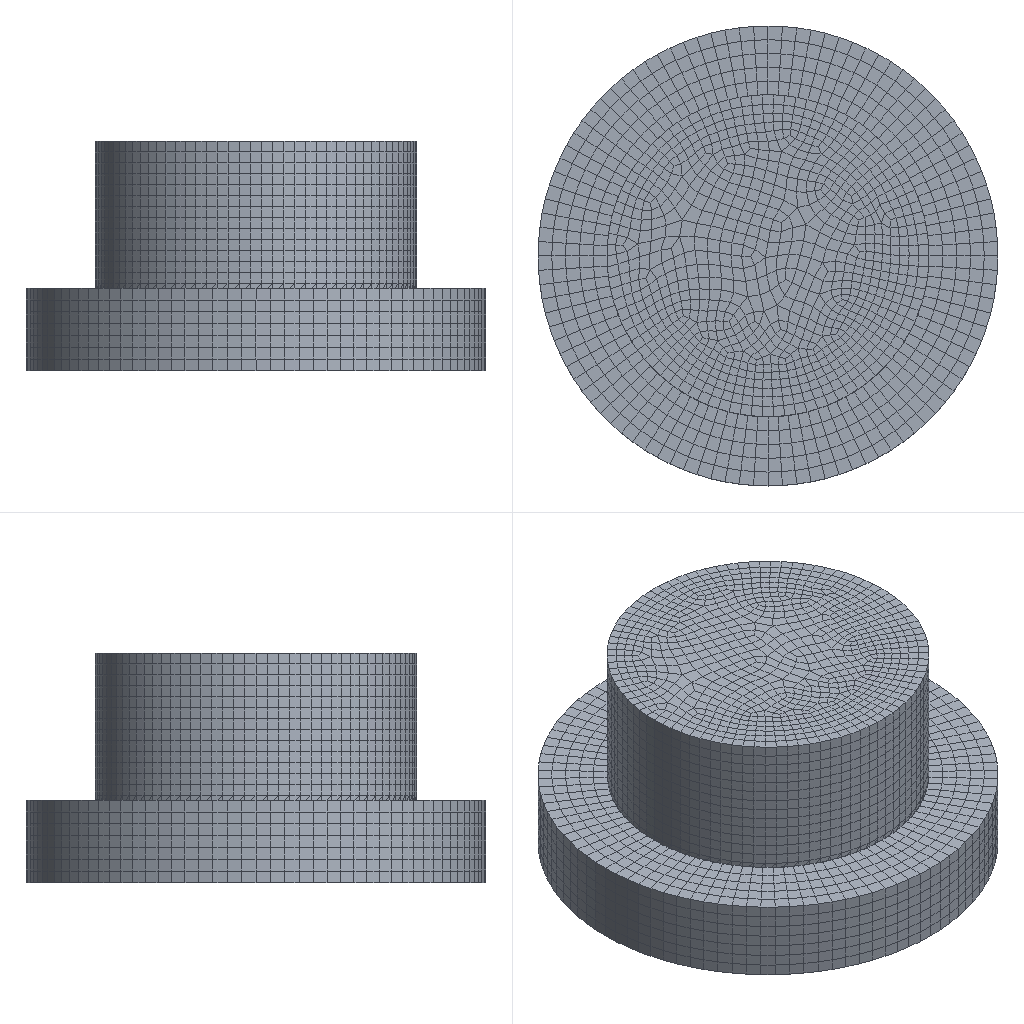Simulation study | ansys workbench
Set-up summary:
category,name,step,type,value,unit,region
solver,ansys_workbench
units,mm-N-s-tonne (MPa),,stated,"/units,MPA"
analysis,LS1,,static
load_step,LS1,LS1,static,nsubst=1; time=1
mesh,nodes,,,96110
mesh,elements,,,24526
element_type,SOLID186,,,21686
element_type,TARGE170,,,1420
element_type,CONTA174,,,1420
material,Aluminum Alloy,,E,71000,tonne s^-2 mm^-1
material,Aluminum Alloy,,nu,0.33
material,Aluminum Alloy,,density,2.77e-09,tonne mm^-3
material,Aluminum Alloy,,conductivity,114
material,Aluminum Alloy,,specific_heat,8.75e+08,mm^2 s^-2 C^-1
material,Aluminum Alloy,,cte,2.3e-05,C^-1
material,Aluminum Alloy,,permeability,1
material,Aluminum Alloy,,resistivity,2.43e-05
material,Structural Steel,,E,200000,tonne s^-2 mm^-1
material,Structural Steel,,nu,0.3
material,Structural Steel,,density,7.85e-09,tonne mm^-3
material,Structural Steel,,conductivity,60.5,tonne mm s^-3 C^-1
material,Structural Steel,,specific_heat,4.34e+08,mm^2 s^-2 C^-1
material,Structural Steel,,cte,1.2e-05,C^-1
material,Structural Steel,,permeability,10000
material,Structural Steel,,resistivity,0.00017,ohm mm
bc,Fixed Supports,model,fixed,[dofs=ALL],,_FIXEDSU
bc,Set Displacements,LS1,prescribed uz,-1 [dofs=UZ],,_CM42UZ_ZP
contact,Frictional - ring To shift,,standard (frictionless/frictional),friction=0.15; element=CONTA174
named_set,_FIXEDSU,,node,1700
named_set,_CM42UZ_ZP,,node,2689
Ansys APDL input file, long lists of numbers shortened:
/batch
/config,noeldb,1     ! force off writing results to database
*get,_wallstrt,active,,time,wall
! ANSYS input file written by Workbench version 19.2 RELEASE
! File used for geometry attach:
/title,[REDACTED]
*DIM,_wb_ProjectScratch_dir,string,248
_wb_ProjectScratch_dir(1) = ''
*DIM,_wb_SolverFiles_dir,string,248
_wb_SolverFiles_dir(1) = ''
*DIM,_wb_userfiles_dir,string,248
_wb_userfiles_dir(1) = ''
/com,--- Data in consistent NMM units. See Solving Units in the help system for more information.
/units,MPA
/nopr
/wb,file,start              !  signify a WB generated input file
/prep7
! Turn off shape checking because checks already performed inside WB mesher.
! See help system for more information.
SHPP,OFF,,NOWARN
/nolist
etcon,set             ! allow ANSYS to choose best KEYOP's for 180x elements
/com,*********** Nodes for the whole assembly ***********
nblock,3,,105721
(1i9,3e20.9e3)
        1     4.700000000E+01     2.351940835E-14     2.571428571E+00
! (96109 more lines like these left out)
-1
/wb,elem,start            !  set before creation of elements
/com,*********** Elements for Body 1 "ring" ***********
et,1,186
keyo,1,2,1          ! set full integration on SOLID186
eblock,19,solid,,3500
(19i9)
        1        1        1        1        0        0        0        0       20        0        1        1       25     4199     4697     2800     2796     4703     4696
! (6999 more lines like these left out)
-1
/com,*********** Elements for Body 2 "shift" ***********
et,2,186
keyo,2,2,1          ! set full integration on SOLID186
eblock,19,solid,,18186
(19i9)
        2        2        2        2        0        0        0        0       20        0     3501    17801    17821    27421    19961    35062    35061    34581    34954
! (36371 more lines like these left out)
-1
/wb,elem,end               !  done creating elements
/com,*********** Send User Defined Coordinate System(s) ***********
csys,0
toffst,273.15,  ! Temperature offset from absolute zero
/com,*********** Set Reference Temperature ***********
tref,22.
/wb,mat,start              !  starting to send materials
/com,*********** Send Materials ***********
Temperature = 'TEMP' ! Temperature
MP,DENS,1,2.77e-09,	! tonne mm^-3
MP,ALPX,1,2.3e-05,	! C^-1
MP,C,1,875000000,	! mm^2 s^-2 C^-1
MPTEMP,,,,,,,,
MPTEMP,1,-100
MPTEMP,2,0
MPTEMP,3,100
MPTEMP,4,200
MPDATA,KXX,1, ,114,144,165,175,	! tonne mm s^-3 C^-1
MPTEMP,,,,,,,,
MPTEMP,,,,,,,,
MPTEMP,1,0
MPTEMP,2,20
MPTEMP,3,100
MPDATA,RSVX,1, ,2.43e-05,2.67e-05,3.63e-05,	! ohm mm
MPTEMP,,,,,,,,
MP,EX,1,71000,	! tonne s^-2 mm^-1
MP,NUXY,1,0.33,
MP,MURX,1,1,
Temperature = 'TEMP' ! Temperature
MP,DENS,2,7.85e-09,	! tonne mm^-3
MP,ALPX,2,1.2e-05,	! C^-1
MP,C,2,434000000,	! mm^2 s^-2 C^-1
MP,KXX,2,60.5,	! tonne mm s^-3 C^-1
MP,RSVX,2,0.00017,	! ohm mm
MP,EX,2,200000,	! tonne s^-2 mm^-1
MP,NUXY,2,0.3,
MP,MURX,2,10000,
/wb,mat,end                !  done sending materials
!************************* Model Summary ********************
!ring,	Aluminum Alloy,	matid,	1
!shift,	Structural Steel,	matid,	2
!************************* End Model Summary ********************
! get the diagonal of the bounding box. Needed later for other things
*get,_xmin,node,,mnloc,x
*get,_ymin,node,,mnloc,y
*get,_zmin,node,,mnloc,z
*get,_xmax,node,,mxloc,x
*get,_ymax,node,,mxloc,y
*get,_zmax,node,,mxloc,z
_ASMDIAG=(_xmax-_xmin)*(_xmax-_xmin)+(_ymax-_ymin)*(_ymax-_ymin)+(_zmax-_zmin)*(_zmax-_zmin)
_ASMDIAG=SQRT(_ASMDIAG)
/wb,contact,start          !  starting to send contact
/com,*********** Create Contact "Frictional - ring To shift" ***********
/com,            Real Constant Set For Above Contact Is 4 & 3
*set,tid,4
*set,cid,3
r,tid
r,cid
et,tid,170
et,cid,174
eblock,10,,,700
(15i9)
    21687        4        4        4        0     3896     3997     3996     3995    16198    16397    16395    16197
! (699 more lines like these left out)
-1
eblock,10,,,700
(15i9)
    22387        3        3        3        0     3896     3997     3996     3995    16198    16397    16395    16197
! (699 more lines like these left out)
-1
eblock,10,,,720
(15i9)
    23087        3        4        3        0    37755    37756    37757    35975    96001    96003    92424    92423
! (719 more lines like these left out)
-1
eblock,10,,,720
(15i9)
    23807        4        3        4        0    37755    37756    37757    35975    96001    96003    92424    92423
! (719 more lines like these left out)
-1
keyo,cid,8,2               ! auto create asymmetric contact (from Program Controlled setting)
keyo,cid,10,0              ! adjust contact stiffness each NR iteration (from Program Controlled setting)
keyo,cid,12,0              ! standard contact
mp,mu,cid,0.15      ! unitless
keyo,cid,18,1              ! small sliding turned on by application
keyo,cid,2,0               ! augmented Lagrange (from Program Controlled setting)
keyo,cid,4,0               ! on Gauss point (from Program Controlled setting)
keyo,cid,9,0               ! use real geometry with stepped effects
keyo,cid,7,0               ! No Prediction
rmod,tid,3,1.       ! FKN
rmod,tid,5,0.       ! ICONT
rmod,tid,6,0.       ! PINB
rmod,tid,10,1.e-002 ! CNOF
rmod,tid,12,0.      ! FKT
rmod,tid,36,27      ! WB DSID
rmod,cid,3,1.       ! FKN
rmod,cid,5,0.       ! ICONT
rmod,cid,6,0.       ! PINB
rmod,cid,10,1.e-002 ! CNOF
rmod,cid,12,0.      ! FKT
rmod,cid,36,27      ! WB DSID
nsel,all
esel,all
/wb,contact,end            !  done creating contacts
/golist
/wb,load,start             !  starting to send loads
/com,*********** Fixed Supports ***********
CMBLOCK,_FIXEDSU,NODE,     1700
(8i10)
      2401      2402      2403      2404      2405      2406      2407      2408
! (212 more lines like these left out)
cmsel,s,_FIXEDSU
d,all,all
nsel,all
/gst,on,on
fini
*get,_numnode,node,0,count
*get,_numelem,elem,0,count
*get, _MAXELEMNUM, elem, 0, NUM, MAX
*get, _MAXNODENUM, node, 0, NUM, MAX
*get, _MAXELEMTYPE, etyp, 0, NUM, MAX
*get, _MAXREALCONST, real, 0, NUM, MAX
/go
/wb,load,end               !  done creating loads
/com,--- Number of total nodes = %_numnode%
/com,--- Number of contact elements = 2840
/com,--- Number of spring elements = 0
/com,--- Number of bearing elements = 0
/com,--- Number of solid elements = 21686
/com,--- Number of condensed parts = 0
/com,--- Number of total elements = %_numelem%
*get,_wallbsol,active,,time,wall
/com,****************************************************************************
/com,*************************    SOLUTION       ********************************
/com,****************************************************************************
/solu
antype,0                   ! static analysis
eqsl,pcg,1e-8,,,,,,1
cntr,print,1               ! print out contact info and also make no initial contact an error
dmpoption,emat,no             ! Don't combine emat file for DANSYS
dmpoption,esav,no             ! Don't combine esav file for DANSYS
nldiag,cont,iter           ! print out contact info each equilibrium iteration
rescontrol,define,last,last,,dele	   ! Program Controlled
/com,****************************************************
/com,******************* SOLVE FOR LS 1 OF 1 ****************
/com,*** Set Displacements ***
CMBLOCK,_CM42UZ_ZP,NODE,     2689
(8i10)
     35063     35064     35065     35066     35067     35068     35069     35070
! (336 more lines like these left out)
cmsel,s,_CM42UZ_ZP
d,all,uz,-1.
nsel,all
/com,*** Component For All Non-Zero UZ Displacements ***
cmsel,s,_CM42uz_zp
cm,_DISPNONZEROUZ,NODE
nsel,all
/nopr
/gopr
autots,on                  ! Workbench Program Controlled automatic time stepping
nsub,1,10,1                ! due to presence of general nonlinear
time,1.
outres,erase
outres,all,none
outres,nsol,all,
outres,rsol,all
outres,strs,all,
outres,epel,all,
outres,eppl,all,
stabilize,off                   ! Stabilization turned OFF by user
! *********** WB SOLVE COMMAND ***********
! check interactive state
*get,ANSINTER_,active,,int
*if,ANSINTER_,ne,0,then
/eof
*endif
solve
/com *************** Write FE CONNECTORS *********
CEWRITE,file,ce,,INTE
/com,****************************************************
/com,*************** FINISHED SOLVE FOR LS 1 *************
*get,_wallasol,active,,time,wall
/nopr
*get,_numnode,node,0,count
*get,_numelem,elem,0,count
*get, _MAXELEMNUM, elem, 0, NUM, MAX
*get, _MAXNODENUM, node, 0, NUM, MAX,,,INTERNAL
*get, _MAXELEMTYPE, etyp, 0, NUM, MAX
*get, _MAXREALCONST, real, 0, NUM, MAX
/gopr
*get,_PCGITER,active,,solu,cgiter
/post1
xmlo,ENCODING,ISO-8859-1
xmlo,parm
/xml,parm,xml
fini
/gopr
*get,_walldone,active,,time,wall
_preptime=(_wallbsol-_wallstrt)*3600
_solvtime=(_wallasol-_wallbsol)*3600
_posttime=(_walldone-_wallasol)*3600
_totaltim=(_walldone-_wallstrt)*3600
/wb,file,end               ! done with WB generated input
Results summary:
result,analyses[0].index,,,1
result,analyses[0].system,,,SYS
result,analyses[0].deck,,,deck.dat
result,analyses[0].solve_status,,,completed
result,analyses[0].analysis_type,,,static
result,analyses[0].physics,,,mechanical
result,analyses[0].unit_system,,,"NMM: mm, ton, N, s, mV, mA, degC"
result,analyses[0].n_sets,,,1
result,analyses[0].load_steps[0].set,set=1,,1
result,analyses[0].load_steps[0].time_or_freq,set=1,,1
result,analyses[0].load_steps[0].max_displacement_magnitude,set=1,,1.002
result,analyses[0].load_steps[0].max_von_mises_nodal,set=1,,159.643
result,analyses[0].load_steps[0].reaction_force_sum_xyz[1],set=1,,-5.40222e-07
result,analyses[0].load_steps[0].reaction_force_sum_xyz[2],set=1,,7.69423e-07
result,analyses[0].load_steps[0].reaction_force_sum_xyz[3],set=1,,-6.259
result,geometry_export[0][0],,,.step
result,geometry_export[0][1],,,ok
result,geometry_export[0][2],,,2